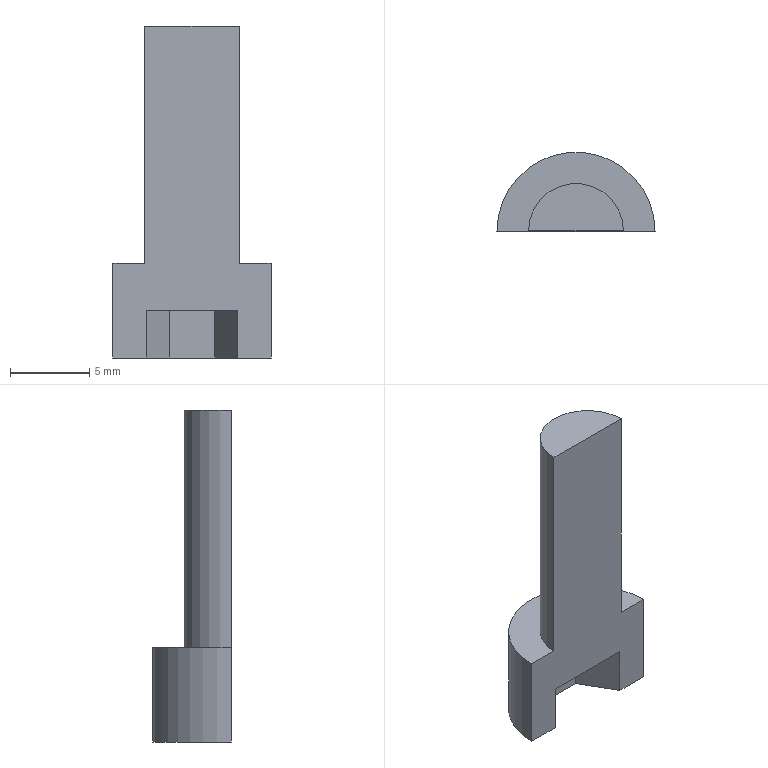Part | STEP file | LG M6_1.5F | 1 solid | 10 faces | box 10 x 5 x 21 mm | volume 414.941 mm3 | plane 8 | cylinder 2 | commonest cylinder face diameters 6 x1 10 x1
STEP:
#1=CARTESIAN_POINT('',(0.,0.,0.));
#2=DIRECTION('',(0.,0.,1.));
#3=DIRECTION('',(1.,0.,0.));
#4=AXIS2_PLACEMENT_3D('',#1,#2,#3);
#5=CARTESIAN_POINT('',(5.,0.,0.));
#6=VERTEX_POINT('',#5);
#7=CARTESIAN_POINT('',(3.,0.,0.));
#8=VERTEX_POINT('',#7);
#9=CARTESIAN_POINT('',(0.,0.,0.));
#10=DIRECTION('',(-1.,0.,0.));
#11=VECTOR('',#10,1.);
#12=LINE('',#9,#11);
#13=CARTESIAN_POINT('',(0.,0.,0.));
#14=DIRECTION('',(0.,0.,1.));
#15=DIRECTION('',(1.,0.,0.));
#16=AXIS2_PLACEMENT_3D('',#13,#14,#15);
#17=PLANE('',#16);
#18=CARTESIAN_POINT('',(0.,0.));
#19=DIRECTION('',(-1.,0.));
#20=VECTOR('',#19,1.);
#21=LINE('',#18,#20);
#22=(GEOMETRIC_REPRESENTATION_CONTEXT(2)PARAMETRIC_REPRESENTATION_CONTEXT()REPRESENTATION_CONTEXT('',''));
#23=DEFINITIONAL_REPRESENTATION('',(#21),#22);
#24=PCURVE('',#17,#23);
#25=CARTESIAN_POINT('',(120.,0.,98.57));
#26=DIRECTION('',(0.,1.,0.));
#27=DIRECTION('',(1.,0.,0.));
#28=AXIS2_PLACEMENT_3D('',#25,#26,#27);
#29=PLANE('',#28);
#30=CARTESIAN_POINT('',(-120.,98.57));
#31=DIRECTION('',(-1.,0.));
#32=VECTOR('',#31,1.);
#33=LINE('',#30,#32);
#34=(GEOMETRIC_REPRESENTATION_CONTEXT(2)PARAMETRIC_REPRESENTATION_CONTEXT()REPRESENTATION_CONTEXT('',''));
#35=DEFINITIONAL_REPRESENTATION('',(#33),#34);
#36=PCURVE('',#29,#35);
#37=SURFACE_CURVE('',#12,(#24,#36),.PCURVE_S1.);
#38=EDGE_CURVE('',#6,#8,#37,.T.);
#39=ORIENTED_EDGE('',*,*,#38,.F.);
#40=CARTESIAN_POINT('',(-5.,0.,0.));
#41=VERTEX_POINT('',#40);
#42=CARTESIAN_POINT('',(0.,0.,0.));
#43=DIRECTION('',(0.,0.,1.));
#44=DIRECTION('',(1.,0.,0.));
#45=AXIS2_PLACEMENT_3D('',#42,#43,#44);
#46=CIRCLE('',#45,5.);
#47=CARTESIAN_POINT('',(0.,0.));
#48=DIRECTION('',(1.,0.));
#49=AXIS2_PLACEMENT_2D('',#47,#48);
#50=CIRCLE('',#49,5.);
#51=(GEOMETRIC_REPRESENTATION_CONTEXT(2)PARAMETRIC_REPRESENTATION_CONTEXT()REPRESENTATION_CONTEXT('',''));
#52=DEFINITIONAL_REPRESENTATION('',(#50),#51);
#53=PCURVE('',#17,#52);
#54=CARTESIAN_POINT('',(0.,0.,-6.));
#55=DIRECTION('',(0.,0.,1.));
#56=DIRECTION('',(1.,0.,0.));
#57=AXIS2_PLACEMENT_3D('',#54,#55,#56);
#58=CYLINDRICAL_SURFACE('',#57,5.);
#59=CARTESIAN_POINT('',(0.,6.));
#60=DIRECTION('',(1.,0.));
#61=VECTOR('',#60,1.);
#62=LINE('',#59,#61);
#63=(GEOMETRIC_REPRESENTATION_CONTEXT(2)PARAMETRIC_REPRESENTATION_CONTEXT()REPRESENTATION_CONTEXT('',''));
#64=DEFINITIONAL_REPRESENTATION('',(#62),#63);
#65=PCURVE('',#58,#64);
#66=SURFACE_CURVE('',#46,(#53,#65),.PCURVE_S1.);
#67=EDGE_CURVE('',#6,#41,#66,.T.);
#68=ORIENTED_EDGE('',*,*,#67,.T.);
#69=CARTESIAN_POINT('',(-3.,0.,0.));
#70=VERTEX_POINT('',#69);
#71=CARTESIAN_POINT('',(0.,0.,0.));
#72=DIRECTION('',(-1.,0.,0.));
#73=VECTOR('',#72,1.);
#74=LINE('',#71,#73);
#75=CARTESIAN_POINT('',(0.,0.));
#76=DIRECTION('',(-1.,0.));
#77=VECTOR('',#76,1.);
#78=LINE('',#75,#77);
#79=(GEOMETRIC_REPRESENTATION_CONTEXT(2)PARAMETRIC_REPRESENTATION_CONTEXT()REPRESENTATION_CONTEXT('',''));
#80=DEFINITIONAL_REPRESENTATION('',(#78),#79);
#81=PCURVE('',#17,#80);
#82=CARTESIAN_POINT('',(-120.,98.57));
#83=DIRECTION('',(-1.,0.));
#84=VECTOR('',#83,1.);
#85=LINE('',#82,#84);
#86=(GEOMETRIC_REPRESENTATION_CONTEXT(2)PARAMETRIC_REPRESENTATION_CONTEXT()REPRESENTATION_CONTEXT('',''));
#87=DEFINITIONAL_REPRESENTATION('',(#85),#86);
#88=PCURVE('',#29,#87);
#89=SURFACE_CURVE('',#74,(#81,#88),.PCURVE_S1.);
#90=EDGE_CURVE('',#70,#41,#89,.T.);
#91=ORIENTED_EDGE('',*,*,#90,.F.);
#92=CARTESIAN_POINT('',(0.,0.,0.));
#93=DIRECTION('',(0.,0.,1.));
#94=DIRECTION('',(1.,0.,0.));
#95=AXIS2_PLACEMENT_3D('',#92,#93,#94);
#96=CIRCLE('',#95,3.);
#97=CARTESIAN_POINT('',(0.,0.));
#98=DIRECTION('',(1.,0.));
#99=AXIS2_PLACEMENT_2D('',#97,#98);
#100=CIRCLE('',#99,3.);
#101=(GEOMETRIC_REPRESENTATION_CONTEXT(2)PARAMETRIC_REPRESENTATION_CONTEXT()REPRESENTATION_CONTEXT('',''));
#102=DEFINITIONAL_REPRESENTATION('',(#100),#101);
#103=PCURVE('',#17,#102);
#104=CARTESIAN_POINT('',(0.,0.,15.));
#105=DIRECTION('',(0.,0.,-1.));
#106=DIRECTION('',(-1.,0.,0.));
#107=AXIS2_PLACEMENT_3D('',#104,#105,#106);
#108=CYLINDRICAL_SURFACE('',#107,3.);
#109=CARTESIAN_POINT('',(3.142,15.));
#110=DIRECTION('',(-1.,0.));
#111=VECTOR('',#110,1.);
#112=LINE('',#109,#111);
#113=(GEOMETRIC_REPRESENTATION_CONTEXT(2)PARAMETRIC_REPRESENTATION_CONTEXT()REPRESENTATION_CONTEXT('',''));
#114=DEFINITIONAL_REPRESENTATION('',(#112),#113);
#115=PCURVE('',#108,#114);
#116=SURFACE_CURVE('',#96,(#103,#115),.PCURVE_S1.);
#117=EDGE_CURVE('',#8,#70,#116,.T.);
#118=ORIENTED_EDGE('',*,*,#117,.F.);
#119=EDGE_LOOP('',(#39,#68,#91,#118));
#120=FACE_BOUND('',#119,.T.);
#121=ADVANCED_FACE('',(#120),#17,.T.);
#122=CARTESIAN_POINT('',(-5.,0.,-6.));
#123=VERTEX_POINT('',#122);
#124=CARTESIAN_POINT('',(-5.,0.,-6.));
#125=DIRECTION('',(0.,0.,-1.));
#126=VECTOR('',#125,1.);
#127=LINE('',#124,#126);
#128=CARTESIAN_POINT('',(3.142,0.));
#129=DIRECTION('',(0.,-1.));
#130=VECTOR('',#129,1.);
#131=LINE('',#128,#130);
#132=(GEOMETRIC_REPRESENTATION_CONTEXT(2)PARAMETRIC_REPRESENTATION_CONTEXT()REPRESENTATION_CONTEXT('',''));
#133=DEFINITIONAL_REPRESENTATION('',(#131),#132);
#134=PCURVE('',#58,#133);
#135=CARTESIAN_POINT('',(-125.,104.57));
#136=DIRECTION('',(0.,1.));
#137=VECTOR('',#136,1.);
#138=LINE('',#135,#137);
#139=(GEOMETRIC_REPRESENTATION_CONTEXT(2)PARAMETRIC_REPRESENTATION_CONTEXT()REPRESENTATION_CONTEXT('',''));
#140=DEFINITIONAL_REPRESENTATION('',(#138),#139);
#141=PCURVE('',#29,#140);
#142=SURFACE_CURVE('',#127,(#134,#141),.PCURVE_S1.);
#143=EDGE_CURVE('',#41,#123,#142,.T.);
#144=ORIENTED_EDGE('',*,*,#143,.F.);
#145=ORIENTED_EDGE('',*,*,#67,.F.);
#146=CARTESIAN_POINT('',(5.,0.,-6.));
#147=VERTEX_POINT('',#146);
#148=CARTESIAN_POINT('',(5.,0.,-6.));
#149=DIRECTION('',(0.,0.,1.));
#150=VECTOR('',#149,1.);
#151=LINE('',#148,#150);
#152=CARTESIAN_POINT('',(0.,0.));
#153=DIRECTION('',(0.,1.));
#154=VECTOR('',#153,1.);
#155=LINE('',#152,#154);
#156=(GEOMETRIC_REPRESENTATION_CONTEXT(2)PARAMETRIC_REPRESENTATION_CONTEXT()REPRESENTATION_CONTEXT('',''));
#157=DEFINITIONAL_REPRESENTATION('',(#155),#156);
#158=PCURVE('',#58,#157);
#159=CARTESIAN_POINT('',(-115.,104.57));
#160=DIRECTION('',(0.,-1.));
#161=VECTOR('',#160,1.);
#162=LINE('',#159,#161);
#163=(GEOMETRIC_REPRESENTATION_CONTEXT(2)PARAMETRIC_REPRESENTATION_CONTEXT()REPRESENTATION_CONTEXT('',''));
#164=DEFINITIONAL_REPRESENTATION('',(#162),#163);
#165=PCURVE('',#29,#164);
#166=SURFACE_CURVE('',#151,(#158,#165),.PCURVE_S1.);
#167=EDGE_CURVE('',#147,#6,#166,.T.);
#168=ORIENTED_EDGE('',*,*,#167,.F.);
#169=CARTESIAN_POINT('',(0.,0.,-6.));
#170=DIRECTION('',(0.,0.,1.));
#171=DIRECTION('',(1.,0.,0.));
#172=AXIS2_PLACEMENT_3D('',#169,#170,#171);
#173=CIRCLE('',#172,5.);
#174=CARTESIAN_POINT('',(0.,0.));
#175=DIRECTION('',(1.,0.));
#176=VECTOR('',#175,1.);
#177=LINE('',#174,#176);
#178=(GEOMETRIC_REPRESENTATION_CONTEXT(2)PARAMETRIC_REPRESENTATION_CONTEXT()REPRESENTATION_CONTEXT('',''));
#179=DEFINITIONAL_REPRESENTATION('',(#177),#178);
#180=PCURVE('',#58,#179);
#181=CARTESIAN_POINT('',(0.,0.,-6.));
#182=DIRECTION('',(0.,0.,1.));
#183=DIRECTION('',(1.,0.,0.));
#184=AXIS2_PLACEMENT_3D('',#181,#182,#183);
#185=PLANE('',#184);
#186=CARTESIAN_POINT('',(0.,0.));
#187=DIRECTION('',(1.,0.));
#188=AXIS2_PLACEMENT_2D('',#186,#187);
#189=CIRCLE('',#188,5.);
#190=(GEOMETRIC_REPRESENTATION_CONTEXT(2)PARAMETRIC_REPRESENTATION_CONTEXT()REPRESENTATION_CONTEXT('',''));
#191=DEFINITIONAL_REPRESENTATION('',(#189),#190);
#192=PCURVE('',#185,#191);
#193=SURFACE_CURVE('',#173,(#180,#192),.PCURVE_S1.);
#194=EDGE_CURVE('',#147,#123,#193,.T.);
#195=ORIENTED_EDGE('',*,*,#194,.T.);
#196=EDGE_LOOP('',(#144,#145,#168,#195));
#197=FACE_BOUND('',#196,.T.);
#198=ADVANCED_FACE('',(#197),#58,.T.);
#199=ORIENTED_EDGE('',*,*,#194,.F.);
#200=CARTESIAN_POINT('',(2.898,0.,-6.));
#201=VERTEX_POINT('',#200);
#202=CARTESIAN_POINT('',(0.,0.,-6.));
#203=DIRECTION('',(-1.,0.,0.));
#204=VECTOR('',#203,1.);
#205=LINE('',#202,#204);
#206=CARTESIAN_POINT('',(0.,0.));
#207=DIRECTION('',(-1.,0.));
#208=VECTOR('',#207,1.);
#209=LINE('',#206,#208);
#210=(GEOMETRIC_REPRESENTATION_CONTEXT(2)PARAMETRIC_REPRESENTATION_CONTEXT()REPRESENTATION_CONTEXT('',''));
#211=DEFINITIONAL_REPRESENTATION('',(#209),#210);
#212=PCURVE('',#185,#211);
#213=CARTESIAN_POINT('',(-120.,104.57));
#214=DIRECTION('',(-1.,0.));
#215=VECTOR('',#214,1.);
#216=LINE('',#213,#215);
#217=(GEOMETRIC_REPRESENTATION_CONTEXT(2)PARAMETRIC_REPRESENTATION_CONTEXT()REPRESENTATION_CONTEXT('',''));
#218=DEFINITIONAL_REPRESENTATION('',(#216),#217);
#219=PCURVE('',#29,#218);
#220=SURFACE_CURVE('',#205,(#212,#219),.PCURVE_S1.);
#221=EDGE_CURVE('',#147,#201,#220,.T.);
#222=ORIENTED_EDGE('',*,*,#221,.T.);
#223=CARTESIAN_POINT('',(1.449,2.51,-6.));
#224=VERTEX_POINT('',#223);
#225=CARTESIAN_POINT('',(1.449,2.51,-6.));
#226=DIRECTION('',(0.5,-0.866,0.));
#227=VECTOR('',#226,1.);
#228=LINE('',#225,#227);
#229=CARTESIAN_POINT('',(1.449,2.51));
#230=DIRECTION('',(0.5,-0.866));
#231=VECTOR('',#230,1.);
#232=LINE('',#229,#231);
#233=(GEOMETRIC_REPRESENTATION_CONTEXT(2)PARAMETRIC_REPRESENTATION_CONTEXT()REPRESENTATION_CONTEXT('',''));
#234=DEFINITIONAL_REPRESENTATION('',(#232),#233);
#235=PCURVE('',#185,#234);
#236=CARTESIAN_POINT('',(1.449,2.51,-3.));
#237=DIRECTION('',(0.866,0.5,0.));
#238=DIRECTION('',(-0.5,0.866,0.));
#239=AXIS2_PLACEMENT_3D('',#236,#237,#238);
#240=PLANE('',#239);
#241=CARTESIAN_POINT('',(0.,-3.));
#242=DIRECTION('',(-1.,0.));
#243=VECTOR('',#242,1.);
#244=LINE('',#241,#243);
#245=(GEOMETRIC_REPRESENTATION_CONTEXT(2)PARAMETRIC_REPRESENTATION_CONTEXT()REPRESENTATION_CONTEXT('',''));
#246=DEFINITIONAL_REPRESENTATION('',(#244),#245);
#247=PCURVE('',#240,#246);
#248=SURFACE_CURVE('',#228,(#235,#247),.PCURVE_S1.);
#249=EDGE_CURVE('',#224,#201,#248,.T.);
#250=ORIENTED_EDGE('',*,*,#249,.F.);
#251=CARTESIAN_POINT('',(-1.449,2.51,-6.));
#252=VERTEX_POINT('',#251);
#253=CARTESIAN_POINT('',(-1.449,2.51,-6.));
#254=DIRECTION('',(1.,0.,0.));
#255=VECTOR('',#254,1.);
#256=LINE('',#253,#255);
#257=CARTESIAN_POINT('',(-1.449,2.51));
#258=DIRECTION('',(1.,0.));
#259=VECTOR('',#258,1.);
#260=LINE('',#257,#259);
#261=(GEOMETRIC_REPRESENTATION_CONTEXT(2)PARAMETRIC_REPRESENTATION_CONTEXT()REPRESENTATION_CONTEXT('',''));
#262=DEFINITIONAL_REPRESENTATION('',(#260),#261);
#263=PCURVE('',#185,#262);
#264=CARTESIAN_POINT('',(-1.449,2.51,-3.));
#265=DIRECTION('',(0.,1.,0.));
#266=DIRECTION('',(0.,0.,1.));
#267=AXIS2_PLACEMENT_3D('',#264,#265,#266);
#268=PLANE('',#267);
#269=CARTESIAN_POINT('',(-3.,0.));
#270=DIRECTION('',(0.,1.));
#271=VECTOR('',#270,1.);
#272=LINE('',#269,#271);
#273=(GEOMETRIC_REPRESENTATION_CONTEXT(2)PARAMETRIC_REPRESENTATION_CONTEXT()REPRESENTATION_CONTEXT('',''));
#274=DEFINITIONAL_REPRESENTATION('',(#272),#273);
#275=PCURVE('',#268,#274);
#276=SURFACE_CURVE('',#256,(#263,#275),.PCURVE_S1.);
#277=EDGE_CURVE('',#252,#224,#276,.T.);
#278=ORIENTED_EDGE('',*,*,#277,.F.);
#279=CARTESIAN_POINT('',(-2.898,0.,-6.));
#280=VERTEX_POINT('',#279);
#281=CARTESIAN_POINT('',(-2.898,0.,-6.));
#282=DIRECTION('',(0.5,0.866,0.));
#283=VECTOR('',#282,1.);
#284=LINE('',#281,#283);
#285=CARTESIAN_POINT('',(-2.898,0.));
#286=DIRECTION('',(0.5,0.866));
#287=VECTOR('',#286,1.);
#288=LINE('',#285,#287);
#289=(GEOMETRIC_REPRESENTATION_CONTEXT(2)PARAMETRIC_REPRESENTATION_CONTEXT()REPRESENTATION_CONTEXT('',''));
#290=DEFINITIONAL_REPRESENTATION('',(#288),#289);
#291=PCURVE('',#185,#290);
#292=CARTESIAN_POINT('',(-2.898,0.,-3.));
#293=DIRECTION('',(-0.866,0.5,0.));
#294=DIRECTION('',(-0.5,-0.866,0.));
#295=AXIS2_PLACEMENT_3D('',#292,#293,#294);
#296=PLANE('',#295);
#297=CARTESIAN_POINT('',(0.,-3.));
#298=DIRECTION('',(-1.,0.));
#299=VECTOR('',#298,1.);
#300=LINE('',#297,#299);
#301=(GEOMETRIC_REPRESENTATION_CONTEXT(2)PARAMETRIC_REPRESENTATION_CONTEXT()REPRESENTATION_CONTEXT('',''));
#302=DEFINITIONAL_REPRESENTATION('',(#300),#301);
#303=PCURVE('',#296,#302);
#304=SURFACE_CURVE('',#284,(#291,#303),.PCURVE_S1.);
#305=EDGE_CURVE('',#280,#252,#304,.T.);
#306=ORIENTED_EDGE('',*,*,#305,.F.);
#307=CARTESIAN_POINT('',(0.,0.,-6.));
#308=DIRECTION('',(-1.,0.,0.));
#309=VECTOR('',#308,1.);
#310=LINE('',#307,#309);
#311=CARTESIAN_POINT('',(0.,0.));
#312=DIRECTION('',(-1.,0.));
#313=VECTOR('',#312,1.);
#314=LINE('',#311,#313);
#315=(GEOMETRIC_REPRESENTATION_CONTEXT(2)PARAMETRIC_REPRESENTATION_CONTEXT()REPRESENTATION_CONTEXT('',''));
#316=DEFINITIONAL_REPRESENTATION('',(#314),#315);
#317=PCURVE('',#185,#316);
#318=CARTESIAN_POINT('',(-120.,104.57));
#319=DIRECTION('',(-1.,0.));
#320=VECTOR('',#319,1.);
#321=LINE('',#318,#320);
#322=(GEOMETRIC_REPRESENTATION_CONTEXT(2)PARAMETRIC_REPRESENTATION_CONTEXT()REPRESENTATION_CONTEXT('',''));
#323=DEFINITIONAL_REPRESENTATION('',(#321),#322);
#324=PCURVE('',#29,#323);
#325=SURFACE_CURVE('',#310,(#317,#324),.PCURVE_S1.);
#326=EDGE_CURVE('',#280,#123,#325,.T.);
#327=ORIENTED_EDGE('',*,*,#326,.T.);
#328=EDGE_LOOP('',(#199,#222,#250,#278,#306,#327));
#329=FACE_BOUND('',#328,.T.);
#330=ADVANCED_FACE('',(#329),#185,.F.);
#331=CARTESIAN_POINT('',(3.,0.,15.));
#332=VERTEX_POINT('',#331);
#333=CARTESIAN_POINT('',(-3.,0.,15.));
#334=VERTEX_POINT('',#333);
#335=CARTESIAN_POINT('',(0.,0.,15.));
#336=DIRECTION('',(0.,0.,1.));
#337=DIRECTION('',(1.,0.,0.));
#338=AXIS2_PLACEMENT_3D('',#335,#336,#337);
#339=CIRCLE('',#338,3.);
#340=CARTESIAN_POINT('',(3.142,0.));
#341=DIRECTION('',(-1.,0.));
#342=VECTOR('',#341,1.);
#343=LINE('',#340,#342);
#344=(GEOMETRIC_REPRESENTATION_CONTEXT(2)PARAMETRIC_REPRESENTATION_CONTEXT()REPRESENTATION_CONTEXT('',''));
#345=DEFINITIONAL_REPRESENTATION('',(#343),#344);
#346=PCURVE('',#108,#345);
#347=CARTESIAN_POINT('',(0.,0.,15.));
#348=DIRECTION('',(0.,0.,1.));
#349=DIRECTION('',(1.,0.,0.));
#350=AXIS2_PLACEMENT_3D('',#347,#348,#349);
#351=PLANE('',#350);
#352=CARTESIAN_POINT('',(0.,0.));
#353=DIRECTION('',(1.,0.));
#354=AXIS2_PLACEMENT_2D('',#352,#353);
#355=CIRCLE('',#354,3.);
#356=(GEOMETRIC_REPRESENTATION_CONTEXT(2)PARAMETRIC_REPRESENTATION_CONTEXT()REPRESENTATION_CONTEXT('',''));
#357=DEFINITIONAL_REPRESENTATION('',(#355),#356);
#358=PCURVE('',#351,#357);
#359=SURFACE_CURVE('',#339,(#346,#358),.PCURVE_S1.);
#360=EDGE_CURVE('',#332,#334,#359,.T.);
#361=ORIENTED_EDGE('',*,*,#360,.F.);
#362=CARTESIAN_POINT('',(3.,0.,15.));
#363=DIRECTION('',(0.,0.,-1.));
#364=VECTOR('',#363,1.);
#365=LINE('',#362,#364);
#366=CARTESIAN_POINT('',(3.142,0.));
#367=DIRECTION('',(0.,1.));
#368=VECTOR('',#367,1.);
#369=LINE('',#366,#368);
#370=(GEOMETRIC_REPRESENTATION_CONTEXT(2)PARAMETRIC_REPRESENTATION_CONTEXT()REPRESENTATION_CONTEXT('',''));
#371=DEFINITIONAL_REPRESENTATION('',(#369),#370);
#372=PCURVE('',#108,#371);
#373=CARTESIAN_POINT('',(-117.,83.57));
#374=DIRECTION('',(0.,1.));
#375=VECTOR('',#374,1.);
#376=LINE('',#373,#375);
#377=(GEOMETRIC_REPRESENTATION_CONTEXT(2)PARAMETRIC_REPRESENTATION_CONTEXT()REPRESENTATION_CONTEXT('',''));
#378=DEFINITIONAL_REPRESENTATION('',(#376),#377);
#379=PCURVE('',#29,#378);
#380=SURFACE_CURVE('',#365,(#372,#379),.PCURVE_S1.);
#381=EDGE_CURVE('',#332,#8,#380,.T.);
#382=ORIENTED_EDGE('',*,*,#381,.T.);
#383=ORIENTED_EDGE('',*,*,#117,.T.);
#384=CARTESIAN_POINT('',(-3.,0.,15.));
#385=DIRECTION('',(0.,0.,1.));
#386=VECTOR('',#385,1.);
#387=LINE('',#384,#386);
#388=CARTESIAN_POINT('',(0.,0.));
#389=DIRECTION('',(0.,-1.));
#390=VECTOR('',#389,1.);
#391=LINE('',#388,#390);
#392=(GEOMETRIC_REPRESENTATION_CONTEXT(2)PARAMETRIC_REPRESENTATION_CONTEXT()REPRESENTATION_CONTEXT('',''));
#393=DEFINITIONAL_REPRESENTATION('',(#391),#392);
#394=PCURVE('',#108,#393);
#395=CARTESIAN_POINT('',(-123.,83.57));
#396=DIRECTION('',(0.,-1.));
#397=VECTOR('',#396,1.);
#398=LINE('',#395,#397);
#399=(GEOMETRIC_REPRESENTATION_CONTEXT(2)PARAMETRIC_REPRESENTATION_CONTEXT()REPRESENTATION_CONTEXT('',''));
#400=DEFINITIONAL_REPRESENTATION('',(#398),#399);
#401=PCURVE('',#29,#400);
#402=SURFACE_CURVE('',#387,(#394,#401),.PCURVE_S1.);
#403=EDGE_CURVE('',#70,#334,#402,.T.);
#404=ORIENTED_EDGE('',*,*,#403,.T.);
#405=EDGE_LOOP('',(#361,#382,#383,#404));
#406=FACE_BOUND('',#405,.T.);
#407=ADVANCED_FACE('',(#406),#108,.T.);
#408=CARTESIAN_POINT('',(0.,0.,15.));
#409=DIRECTION('',(-1.,0.,0.));
#410=VECTOR('',#409,1.);
#411=LINE('',#408,#410);
#412=CARTESIAN_POINT('',(0.,0.));
#413=DIRECTION('',(-1.,0.));
#414=VECTOR('',#413,1.);
#415=LINE('',#412,#414);
#416=(GEOMETRIC_REPRESENTATION_CONTEXT(2)PARAMETRIC_REPRESENTATION_CONTEXT()REPRESENTATION_CONTEXT('',''));
#417=DEFINITIONAL_REPRESENTATION('',(#415),#416);
#418=PCURVE('',#351,#417);
#419=CARTESIAN_POINT('',(-120.,83.57));
#420=DIRECTION('',(-1.,0.));
#421=VECTOR('',#420,1.);
#422=LINE('',#419,#421);
#423=(GEOMETRIC_REPRESENTATION_CONTEXT(2)PARAMETRIC_REPRESENTATION_CONTEXT()REPRESENTATION_CONTEXT('',''));
#424=DEFINITIONAL_REPRESENTATION('',(#422),#423);
#425=PCURVE('',#29,#424);
#426=SURFACE_CURVE('',#411,(#418,#425),.PCURVE_S1.);
#427=EDGE_CURVE('',#332,#334,#426,.T.);
#428=ORIENTED_EDGE('',*,*,#427,.F.);
#429=ORIENTED_EDGE('',*,*,#360,.T.);
#430=EDGE_LOOP('',(#428,#429));
#431=FACE_BOUND('',#430,.T.);
#432=ADVANCED_FACE('',(#431),#351,.T.);
#433=ORIENTED_EDGE('',*,*,#249,.T.);
#434=CARTESIAN_POINT('',(2.898,0.,-3.));
#435=VERTEX_POINT('',#434);
#436=CARTESIAN_POINT('',(2.898,0.,-3.));
#437=DIRECTION('',(0.,0.,-1.));
#438=VECTOR('',#437,1.);
#439=LINE('',#436,#438);
#440=CARTESIAN_POINT('',(-2.898,0.));
#441=DIRECTION('',(0.,-1.));
#442=VECTOR('',#441,1.);
#443=LINE('',#440,#442);
#444=(GEOMETRIC_REPRESENTATION_CONTEXT(2)PARAMETRIC_REPRESENTATION_CONTEXT()REPRESENTATION_CONTEXT('',''));
#445=DEFINITIONAL_REPRESENTATION('',(#443),#444);
#446=PCURVE('',#240,#445);
#447=CARTESIAN_POINT('',(-117.102,101.57));
#448=DIRECTION('',(0.,1.));
#449=VECTOR('',#448,1.);
#450=LINE('',#447,#449);
#451=(GEOMETRIC_REPRESENTATION_CONTEXT(2)PARAMETRIC_REPRESENTATION_CONTEXT()REPRESENTATION_CONTEXT('',''));
#452=DEFINITIONAL_REPRESENTATION('',(#450),#451);
#453=PCURVE('',#29,#452);
#454=SURFACE_CURVE('',#439,(#446,#453),.PCURVE_S1.);
#455=EDGE_CURVE('',#435,#201,#454,.T.);
#456=ORIENTED_EDGE('',*,*,#455,.F.);
#457=CARTESIAN_POINT('',(1.449,2.51,-3.));
#458=VERTEX_POINT('',#457);
#459=CARTESIAN_POINT('',(1.449,2.51,-3.));
#460=DIRECTION('',(0.5,-0.866,0.));
#461=VECTOR('',#460,1.);
#462=LINE('',#459,#461);
#463=CARTESIAN_POINT('',(0.,0.));
#464=DIRECTION('',(-1.,0.));
#465=VECTOR('',#464,1.);
#466=LINE('',#463,#465);
#467=(GEOMETRIC_REPRESENTATION_CONTEXT(2)PARAMETRIC_REPRESENTATION_CONTEXT()REPRESENTATION_CONTEXT('',''));
#468=DEFINITIONAL_REPRESENTATION('',(#466),#467);
#469=PCURVE('',#240,#468);
#470=CARTESIAN_POINT('',(0.,0.,-3.));
#471=DIRECTION('',(0.,0.,-1.));
#472=DIRECTION('',(-1.,0.,0.));
#473=AXIS2_PLACEMENT_3D('',#470,#471,#472);
#474=PLANE('',#473);
#475=CARTESIAN_POINT('',(-1.449,2.51));
#476=DIRECTION('',(-0.5,-0.866));
#477=VECTOR('',#476,1.);
#478=LINE('',#475,#477);
#479=(GEOMETRIC_REPRESENTATION_CONTEXT(2)PARAMETRIC_REPRESENTATION_CONTEXT()REPRESENTATION_CONTEXT('',''));
#480=DEFINITIONAL_REPRESENTATION('',(#478),#479);
#481=PCURVE('',#474,#480);
#482=SURFACE_CURVE('',#462,(#469,#481),.PCURVE_S1.);
#483=EDGE_CURVE('',#458,#435,#482,.T.);
#484=ORIENTED_EDGE('',*,*,#483,.F.);
#485=CARTESIAN_POINT('',(1.449,2.51,-3.));
#486=DIRECTION('',(0.,0.,-1.));
#487=VECTOR('',#486,1.);
#488=LINE('',#485,#487);
#489=CARTESIAN_POINT('',(0.,0.));
#490=DIRECTION('',(0.,-1.));
#491=VECTOR('',#490,1.);
#492=LINE('',#489,#491);
#493=(GEOMETRIC_REPRESENTATION_CONTEXT(2)PARAMETRIC_REPRESENTATION_CONTEXT()REPRESENTATION_CONTEXT('',''));
#494=DEFINITIONAL_REPRESENTATION('',(#492),#493);
#495=PCURVE('',#240,#494);
#496=CARTESIAN_POINT('',(0.,2.898));
#497=DIRECTION('',(-1.,0.));
#498=VECTOR('',#497,1.);
#499=LINE('',#496,#498);
#500=(GEOMETRIC_REPRESENTATION_CONTEXT(2)PARAMETRIC_REPRESENTATION_CONTEXT()REPRESENTATION_CONTEXT('',''));
#501=DEFINITIONAL_REPRESENTATION('',(#499),#500);
#502=PCURVE('',#268,#501);
#503=SURFACE_CURVE('',#488,(#495,#502),.PCURVE_S1.);
#504=EDGE_CURVE('',#458,#224,#503,.T.);
#505=ORIENTED_EDGE('',*,*,#504,.T.);
#506=EDGE_LOOP('',(#433,#456,#484,#505));
#507=FACE_BOUND('',#506,.T.);
#508=ADVANCED_FACE('',(#507),#240,.F.);
#509=ORIENTED_EDGE('',*,*,#277,.T.);
#510=ORIENTED_EDGE('',*,*,#504,.F.);
#511=CARTESIAN_POINT('',(-1.449,2.51,-3.));
#512=VERTEX_POINT('',#511);
#513=CARTESIAN_POINT('',(-1.449,2.51,-3.));
#514=DIRECTION('',(1.,0.,0.));
#515=VECTOR('',#514,1.);
#516=LINE('',#513,#515);
#517=CARTESIAN_POINT('',(0.,0.));
#518=DIRECTION('',(0.,1.));
#519=VECTOR('',#518,1.);
#520=LINE('',#517,#519);
#521=(GEOMETRIC_REPRESENTATION_CONTEXT(2)PARAMETRIC_REPRESENTATION_CONTEXT()REPRESENTATION_CONTEXT('',''));
#522=DEFINITIONAL_REPRESENTATION('',(#520),#521);
#523=PCURVE('',#268,#522);
#524=CARTESIAN_POINT('',(1.449,2.51));
#525=DIRECTION('',(-1.,0.));
#526=VECTOR('',#525,1.);
#527=LINE('',#524,#526);
#528=(GEOMETRIC_REPRESENTATION_CONTEXT(2)PARAMETRIC_REPRESENTATION_CONTEXT()REPRESENTATION_CONTEXT('',''));
#529=DEFINITIONAL_REPRESENTATION('',(#527),#528);
#530=PCURVE('',#474,#529);
#531=SURFACE_CURVE('',#516,(#523,#530),.PCURVE_S1.);
#532=EDGE_CURVE('',#512,#458,#531,.T.);
#533=ORIENTED_EDGE('',*,*,#532,.F.);
#534=CARTESIAN_POINT('',(-1.449,2.51,-3.));
#535=DIRECTION('',(0.,0.,-1.));
#536=VECTOR('',#535,1.);
#537=LINE('',#534,#536);
#538=CARTESIAN_POINT('',(0.,0.));
#539=DIRECTION('',(-1.,0.));
#540=VECTOR('',#539,1.);
#541=LINE('',#538,#540);
#542=(GEOMETRIC_REPRESENTATION_CONTEXT(2)PARAMETRIC_REPRESENTATION_CONTEXT()REPRESENTATION_CONTEXT('',''));
#543=DEFINITIONAL_REPRESENTATION('',(#541),#542);
#544=PCURVE('',#268,#543);
#545=CARTESIAN_POINT('',(-2.898,0.));
#546=DIRECTION('',(0.,-1.));
#547=VECTOR('',#546,1.);
#548=LINE('',#545,#547);
#549=(GEOMETRIC_REPRESENTATION_CONTEXT(2)PARAMETRIC_REPRESENTATION_CONTEXT()REPRESENTATION_CONTEXT('',''));
#550=DEFINITIONAL_REPRESENTATION('',(#548),#549);
#551=PCURVE('',#296,#550);
#552=SURFACE_CURVE('',#537,(#544,#551),.PCURVE_S1.);
#553=EDGE_CURVE('',#512,#252,#552,.T.);
#554=ORIENTED_EDGE('',*,*,#553,.T.);
#555=EDGE_LOOP('',(#509,#510,#533,#554));
#556=FACE_BOUND('',#555,.T.);
#557=ADVANCED_FACE('',(#556),#268,.F.);
#558=ORIENTED_EDGE('',*,*,#305,.T.);
#559=ORIENTED_EDGE('',*,*,#553,.F.);
#560=CARTESIAN_POINT('',(-2.898,0.,-3.));
#561=VERTEX_POINT('',#560);
#562=CARTESIAN_POINT('',(-2.898,0.,-3.));
#563=DIRECTION('',(0.5,0.866,0.));
#564=VECTOR('',#563,1.);
#565=LINE('',#562,#564);
#566=CARTESIAN_POINT('',(0.,0.));
#567=DIRECTION('',(-1.,0.));
#568=VECTOR('',#567,1.);
#569=LINE('',#566,#568);
#570=(GEOMETRIC_REPRESENTATION_CONTEXT(2)PARAMETRIC_REPRESENTATION_CONTEXT()REPRESENTATION_CONTEXT('',''));
#571=DEFINITIONAL_REPRESENTATION('',(#569),#570);
#572=PCURVE('',#296,#571);
#573=CARTESIAN_POINT('',(2.898,0.));
#574=DIRECTION('',(-0.5,0.866));
#575=VECTOR('',#574,1.);
#576=LINE('',#573,#575);
#577=(GEOMETRIC_REPRESENTATION_CONTEXT(2)PARAMETRIC_REPRESENTATION_CONTEXT()REPRESENTATION_CONTEXT('',''));
#578=DEFINITIONAL_REPRESENTATION('',(#576),#577);
#579=PCURVE('',#474,#578);
#580=SURFACE_CURVE('',#565,(#572,#579),.PCURVE_S1.);
#581=EDGE_CURVE('',#561,#512,#580,.T.);
#582=ORIENTED_EDGE('',*,*,#581,.F.);
#583=CARTESIAN_POINT('',(-2.898,0.,-3.));
#584=DIRECTION('',(0.,0.,-1.));
#585=VECTOR('',#584,1.);
#586=LINE('',#583,#585);
#587=CARTESIAN_POINT('',(0.,0.));
#588=DIRECTION('',(0.,-1.));
#589=VECTOR('',#588,1.);
#590=LINE('',#587,#589);
#591=(GEOMETRIC_REPRESENTATION_CONTEXT(2)PARAMETRIC_REPRESENTATION_CONTEXT()REPRESENTATION_CONTEXT('',''));
#592=DEFINITIONAL_REPRESENTATION('',(#590),#591);
#593=PCURVE('',#296,#592);
#594=CARTESIAN_POINT('',(-122.898,101.57));
#595=DIRECTION('',(0.,1.));
#596=VECTOR('',#595,1.);
#597=LINE('',#594,#596);
#598=(GEOMETRIC_REPRESENTATION_CONTEXT(2)PARAMETRIC_REPRESENTATION_CONTEXT()REPRESENTATION_CONTEXT('',''));
#599=DEFINITIONAL_REPRESENTATION('',(#597),#598);
#600=PCURVE('',#29,#599);
#601=SURFACE_CURVE('',#586,(#593,#600),.PCURVE_S1.);
#602=EDGE_CURVE('',#561,#280,#601,.T.);
#603=ORIENTED_EDGE('',*,*,#602,.T.);
#604=EDGE_LOOP('',(#558,#559,#582,#603));
#605=FACE_BOUND('',#604,.T.);
#606=ADVANCED_FACE('',(#605),#296,.F.);
#607=CARTESIAN_POINT('',(0.,0.,-3.));
#608=DIRECTION('',(1.,0.,0.));
#609=VECTOR('',#608,1.);
#610=LINE('',#607,#609);
#611=CARTESIAN_POINT('',(0.,0.));
#612=DIRECTION('',(-1.,0.));
#613=VECTOR('',#612,1.);
#614=LINE('',#611,#613);
#615=(GEOMETRIC_REPRESENTATION_CONTEXT(2)PARAMETRIC_REPRESENTATION_CONTEXT()REPRESENTATION_CONTEXT('',''));
#616=DEFINITIONAL_REPRESENTATION('',(#614),#615);
#617=PCURVE('',#474,#616);
#618=CARTESIAN_POINT('',(-120.,101.57));
#619=DIRECTION('',(1.,0.));
#620=VECTOR('',#619,1.);
#621=LINE('',#618,#620);
#622=(GEOMETRIC_REPRESENTATION_CONTEXT(2)PARAMETRIC_REPRESENTATION_CONTEXT()REPRESENTATION_CONTEXT('',''));
#623=DEFINITIONAL_REPRESENTATION('',(#621),#622);
#624=PCURVE('',#29,#623);
#625=SURFACE_CURVE('',#610,(#617,#624),.PCURVE_S1.);
#626=EDGE_CURVE('',#561,#435,#625,.T.);
#627=ORIENTED_EDGE('',*,*,#626,.F.);
#628=ORIENTED_EDGE('',*,*,#581,.T.);
#629=ORIENTED_EDGE('',*,*,#532,.T.);
#630=ORIENTED_EDGE('',*,*,#483,.T.);
#631=EDGE_LOOP('',(#627,#628,#629,#630));
#632=FACE_BOUND('',#631,.T.);
#633=ADVANCED_FACE('',(#632),#474,.T.);
#634=ORIENTED_EDGE('',*,*,#167,.T.);
#635=ORIENTED_EDGE('',*,*,#38,.T.);
#636=ORIENTED_EDGE('',*,*,#381,.F.);
#637=ORIENTED_EDGE('',*,*,#427,.T.);
#638=ORIENTED_EDGE('',*,*,#403,.F.);
#639=ORIENTED_EDGE('',*,*,#90,.T.);
#640=ORIENTED_EDGE('',*,*,#143,.T.);
#641=ORIENTED_EDGE('',*,*,#326,.F.);
#642=ORIENTED_EDGE('',*,*,#602,.F.);
#643=ORIENTED_EDGE('',*,*,#626,.T.);
#644=ORIENTED_EDGE('',*,*,#455,.T.);
#645=ORIENTED_EDGE('',*,*,#221,.F.);
#646=EDGE_LOOP('',(#634,#635,#636,#637,#638,#639,#640,#641,#642,#643,#644,#645));
#647=FACE_BOUND('',#646,.T.);
#648=ADVANCED_FACE('',(#647),#29,.F.);
#649=CLOSED_SHELL('',(#121,#198,#330,#407,#432,#508,#557,#606,#633,#648));
#650=MANIFOLD_SOLID_BREP('',#649);
#651=(LENGTH_UNIT()NAMED_UNIT(*)SI_UNIT(.MILLI.,.METRE.));
#652=UNCERTAINTY_MEASURE_WITH_UNIT(LENGTH_MEASURE(0.0000001),#651,'','');
#653=(NAMED_UNIT(*)PLANE_ANGLE_UNIT()SI_UNIT($,.RADIAN.));
#654=(NAMED_UNIT(*)SI_UNIT($,.STERADIAN.)SOLID_ANGLE_UNIT());
#655=(GEOMETRIC_REPRESENTATION_CONTEXT(3)GLOBAL_UNCERTAINTY_ASSIGNED_CONTEXT((#652))GLOBAL_UNIT_ASSIGNED_CONTEXT((#651,#653,#654))REPRESENTATION_CONTEXT('',''));
#656=ADVANCED_BREP_SHAPE_REPRESENTATION('',(#4,#650),#655);